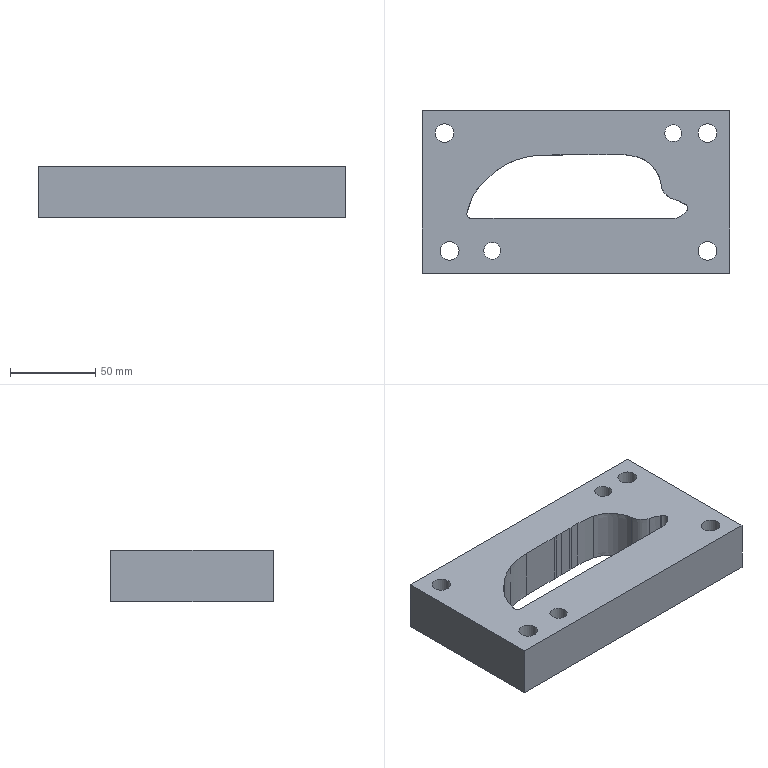Part | STEP file | 208_id710_x_t | 1 solid | 49 faces | box 180 x 95 x 30 mm | volume 370970 mm3 | cylinder 17 | other 17 | plane 15 | commonest cylinder face diameters 11 x6 5 x4 17 x4 10 x2 20 x1